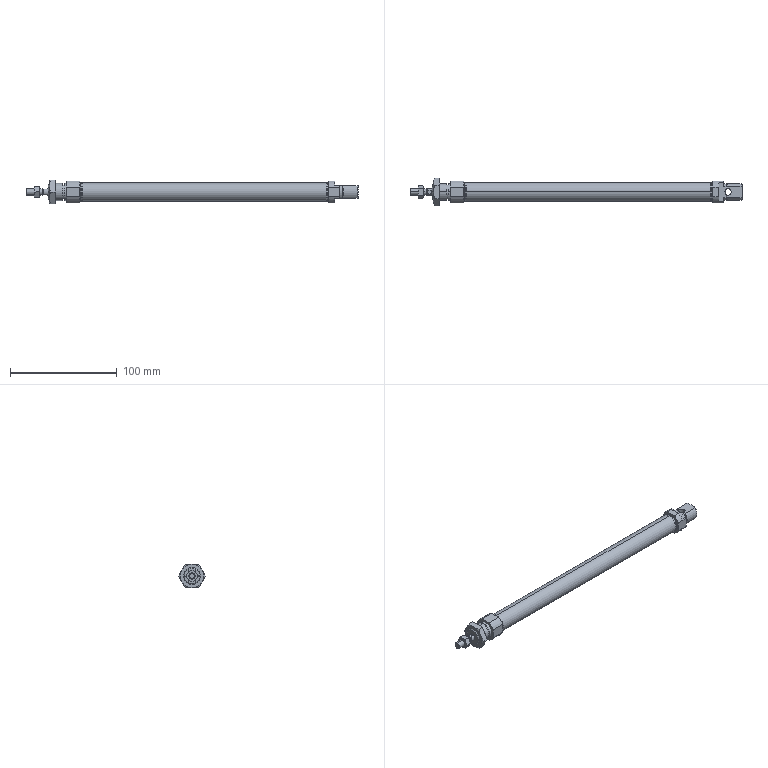Part | STEP file | pen-type cylinder MI16x200SCA | 4 solids | 160 faces | box 311 x 25.403 x 22 mm | volume 38961 mm3 | plane 56 | cylinder 50 | cone 46 | spline 8 | commonest cylinder face diameters 6 x8 16 x8 22 x8 17.4 x6 4.134 x4 14 x4